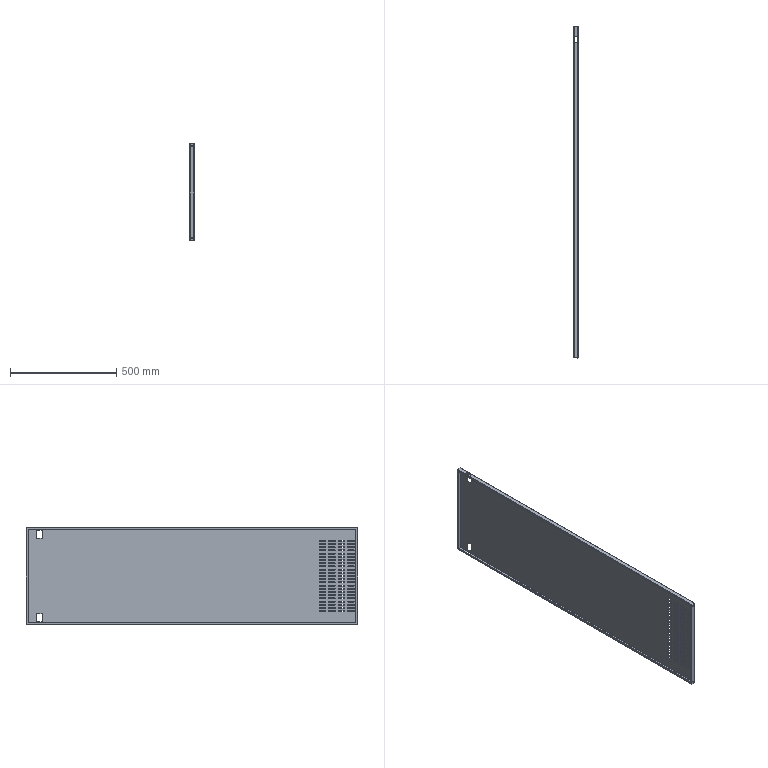Part | SolidWorks | features SplitBody 1 | 1 solid | 458 faces | box 20 x 1560 x 458 mm | volume 808412 mm3 | plane 236 | cylinder 206 | spline 16 | commonest cylinder face diameters 5 x184 0.2 x10 2.2 x8 4.5 x4